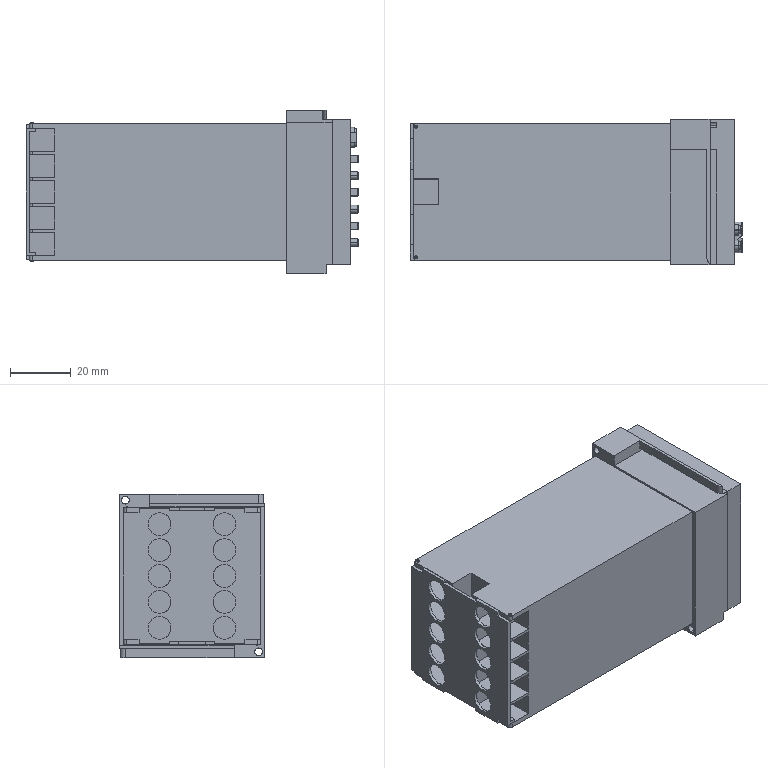Part | STEP file | Omron | 7 solids | 647 faces | box 109 x 47.8 x 53.73 mm | volume 203116 mm3 | plane 388 | cylinder 162 | torus 56 | spline 29 | sphere 12 | commonest cylinder face diameters 0.2 x56 2.5 x24 7.5 x20 2 x12 2.7 x12 0.9 x8